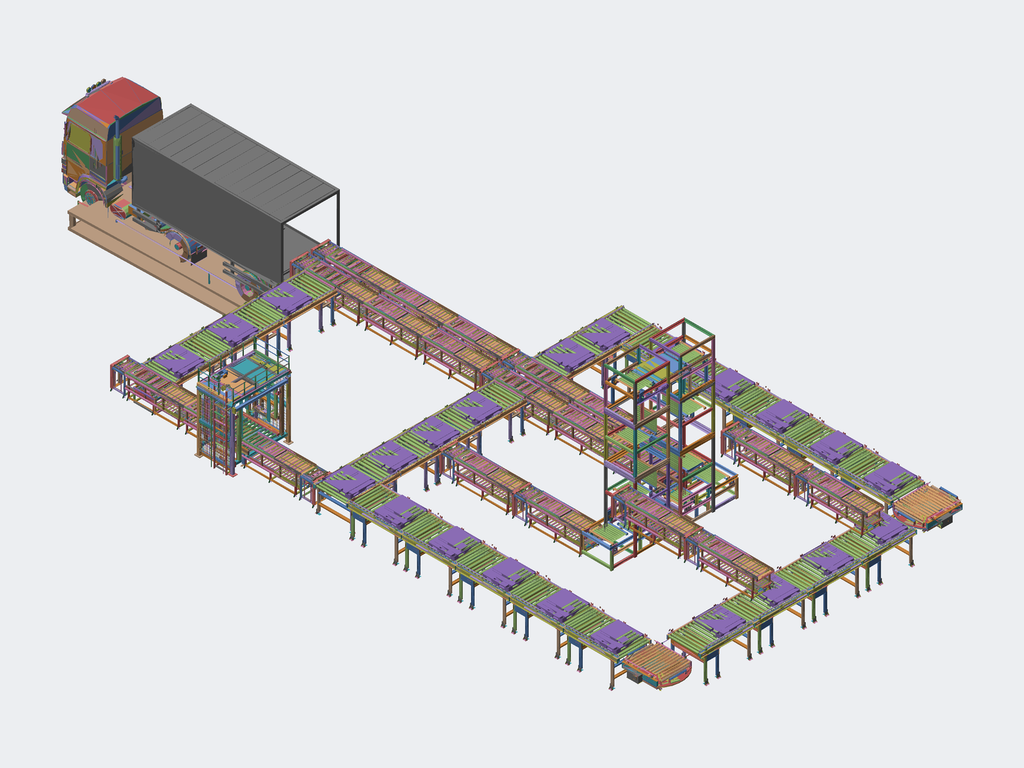Assembly | STEP file | 551 different items | 36567 placed
Parts list (item | name | quantity | parent item | size | volume), first 334 of 551 items:
1 | Sprocket mounting plate XG | x12 | in Single sprocket assembly 1XG(default), Single sprocket assembly 1XG(default)-1, Single sprocket assembly 1XG(default-_flexible1), Single sprocket assembly 1XG(default)-2, Single sprocket assembly 2XG, Single sprocket assembly 2XG-1 | 190 x 350 x 25 mm | 1631084 mm3
2 | 24A16T sprocket XG | x12 | in Single sprocket assembly 1XG(default), Single sprocket assembly 1XG(default)-1, Single sprocket assembly 1XG(default-_flexible1), Single sprocket assembly 1XG(default)-2, Single sprocket assembly 2XG, Single sprocket assembly 2XG-1 | 210 x 210 x 50 mm | 700498 mm3
3 | Single sprocket shaft 1XG | x8 | in Single sprocket assembly 1XG(default), Single sprocket assembly 1XG(default)-1, Single sprocket assembly 1XG(default-_flexible1), Single sprocket assembly 1XG(default)-2 | 50 x 60 x 140 mm | 188778 mm3
4 | 6208 deep groove ball bearing XG | x24 | in Single sprocket assembly 1XG(default), Single sprocket assembly 1XG(default)-1, Single sprocket assembly 1XG(default-_flexible1), Single sprocket assembly 1XG(default)-2, Single sprocket assembly 2XG, Single sprocket assembly 2XG-1 | - | -
5 | Single sprocket shaft end cover 1XG | x12 | in Single sprocket assembly 1XG(default), Single sprocket assembly 1XG(default)-1, Single sprocket assembly 1XG(default-_flexible1), Single sprocket assembly 1XG(default)-2, Single sprocket assembly 2XG, Single sprocket assembly 2XG-1 | 60 x 60 x 10 mm | 27505 mm3
6 | 40 spacer XG | x12 | in Single sprocket assembly 1XG(default), Single sprocket assembly 1XG(default)-1, Single sprocket assembly 1XG(default-_flexible1), Single sprocket assembly 1XG(default)-2, Single sprocket assembly 2XG, Single sprocket assembly 2XG-1 | 70 x 70 x 5 mm | 12959 mm3
7 | Single sprocket shaft 2XG | x4 | in Single sprocket assembly 2XG, Single sprocket assembly 2XG-1 | 80 x 80 x 230 mm | 591587 mm3
8 | Bearing housing mounting plate XG | x12 | in Double sprocket bearing housing assembly 1XG, Double sprocket bearing housing assembly 1XG-1, Double sprocket bearing housing assembly 1XG-2, Double sprocket bearing housing assembly 1XG-3, Double sprocket bearing housing assembly 1XG-4, Double sprocket bearing housing assembly 1XG-5 | 190 x 350 x 25 mm | 1489768 mm3
9 | UCF208 bearing housing XG | x12 | in Double sprocket bearing housing assembly 1XG, Double sprocket bearing housing assembly 1XG-1, Double sprocket bearing housing assembly 1XG-2, Double sprocket bearing housing assembly 1XG-3, Double sprocket bearing housing assembly 1XG-4, Double sprocket bearing housing assembly 1XG-5 | 130 x 130 x 51.2 mm | 310699 mm3
10 | Drive double sprocket shaft 1XG | x4 | in Drive double sprocket assembly 1XG, Drive double sprocket assembly 1XG-1 | 50 x 50 x 1380 mm | 2550231 mm3
11 | 24A16T sprocket 2XG | x24 | in Drive double sprocket assembly 1XG, Double sprocket assembly 1XG, Drive double sprocket assembly 1XG-1 | 210 x 210 x 50 mm | 809619 mm3
12 | 40 bushing | x12 | in Drive double sprocket assembly 1XG, Double sprocket assembly 1XG, Drive double sprocket assembly 1XG-1 | 90 x 90 x 40 mm | 139406 mm3
13 | Double sprocket shaft 1XG | x2 | in Double sprocket assembly 1XG | 50 x 50 x 1320 mm | 2495026 mm3
14 | Outer chain 1XG | x4 | in Outer chain assembly 1XG, Outer chain assembly 1XG-1 | - | 6318542 mm3
15 | Outer chain 1-1XG | x4 | in Outer chain assembly 1XG, Outer chain assembly 1XG-1 | - | 4555438 mm3
16 | Inner chain 1XG | x4 | in Inner chain assembly 1XG, Inner chain assembly 1XG-1 | - | 4855051 mm3
17 | Inner chain 1-1XG | x4 | in Inner chain assembly 1XG, Inner chain assembly 1XG-1 | - | 4555438 mm3
18 | 24A double-side double-hole chain 1 | x420 | in Double-side double-hole chain assembly 1, Double-side double-hole chain assembly 1-1, Double-side double-hole chain assembly 1-2, Double-side double-hole chain assembly 1-3, Double-side double-hole chain assembly 1-4, Double-side double-hole chain assembly 1-5, Double-side double-hole chain assembly 1-6, Double-side double-hole chain assembly 1-7, Double-side double-hole chain assembly 1-8, Double-side double-hole chain assembly 1-9, Double-side double-hole chain assembly 1-10, Double-side double-hole chain assembly 1-11, Double-side double-hole chain assembly 1-12, Double-side double-hole chain assembly 1-13, Double-side double-hole chain assembly 1-14, Double-side double-hole chain assembly 1-15, Double-side double-hole chain assembly 1-16, Double-side double-hole chain assembly 1-17, Double-side double-hole chain assembly 1-18, Double-side double-hole chain assembly 1-19, Double-side double-hole chain assembly 1-20 | 68 x 38 x 99 mm | 48081 mm3
19 | 24A double-side double-hole chain 2 | x378 | in Double-side double-hole chain assembly 1, Double-side double-hole chain assembly 1-1, Double-side double-hole chain assembly 1-2, Double-side double-hole chain assembly 1-3, Double-side double-hole chain assembly 1-4, Double-side double-hole chain assembly 1-5, Double-side double-hole chain assembly 1-6, Double-side double-hole chain assembly 1-7, Double-side double-hole chain assembly 1-8, Double-side double-hole chain assembly 1-9, Double-side double-hole chain assembly 1-10, Double-side double-hole chain assembly 1-11, Double-side double-hole chain assembly 1-12, Double-side double-hole chain assembly 1-13, Double-side double-hole chain assembly 1-14, Double-side double-hole chain assembly 1-15, Double-side double-hole chain assembly 1-16, Double-side double-hole chain assembly 1-17, Double-side double-hole chain assembly 1-18, Double-side double-hole chain assembly 1-19, Double-side double-hole chain assembly 1-20 | 73 x 35 x 35 mm | 33789 mm3
20 | Rear link plate | x14 | in Link plate assembly, 链PlateAssembly-1, 链PlateAssembly-2, 链PlateAssembly-3, 链PlateAssembly-4, 链PlateAssembly-5, 链PlateAssembly-6 | 68 x 70 x 1000 mm | 1230922 mm3
21 | Front link plate | x14 | in Link plate assembly, 链PlateAssembly-1, 链PlateAssembly-2, 链PlateAssembly-3, 链PlateAssembly-4, 链PlateAssembly-5, 链PlateAssembly-6 | 68 x 70 x 820 mm | 1047322 mm3
22 | Middle link plate | x112 | in Link plate assembly, 链PlateAssembly-1, 链PlateAssembly-2, 链PlateAssembly-3, 链PlateAssembly-4, 链PlateAssembly-5, 链PlateAssembly-6 | 74 x 15 x 820 mm | 903391 mm3
23 | Conveyor belt bracket | x4 | in Conveyor assembly 1 | 63 x 160 x 1184 mm | 2475798 mm3
24 | Adjusting plate XG | x4 | in Conveyor assembly 1 | 450 x 110 x 10 mm | 387044 mm3
25 | Bearing mounting plate XG | x4 | in Conveyor assembly 1 | 132 x 110 x 25 mm | 218118 mm3
26 | Adjusting plate-1XG | x4 | in Conveyor assembly 1 | 300 x 110 x 55 mm | 464863 mm3
27 | Screw seat XG | x4 | in Conveyor assembly 1 | 90 x 60 x 60 mm | 144633 mm3
28 | Adjusting plate clamp | x4 | in Conveyor assembly 1 | 30 x 110 x 10 mm | 31099 mm3
29 | Bearing housing F206 | x8 | in Conveyor assembly 1 | 106 x 41.5 x 106 mm | 142901 mm3
30 | socket head cap screw_iso(ISO 4762 M10 x 40 - 40N) | x4 | in Conveyor assembly 1 | 50 x 16 x 16 mm | 4794 mm3
31 | Roller XG3 | x2 | in Conveyor assembly 1 | 175 x 250 x 175 mm | 677038 mm3
32 | Roller XG1 | x4 | in Conveyor assembly 1 | 195 x 987 x 195 mm | 5708379 mm3
33 | Roller XG2 | x6 | in Conveyor assembly 1 | 175 x 105 x 175 mm | 577278 mm3
34 | Belt XG | x2 | in Conveyor assembly 1 | 1201 x 201 x 950 mm | 7472801 mm3
35 | Reinforcing rod XG | x4 | in Conveyor assembly 1 | 110 x 1000 x 60 mm | 1058206 mm3
36 | Bracket 1XG(default_machined_) | x2 | in Continuous lifting machine assembly 1XG | 2500 x 1300 x 2850 mm | 65972501 mm3
37 | Bracket 2XG(default_machined_) | x2 | in Continuous lifting machine assembly 1XG | 1500 x 1300 x 1950 mm | 30079515 mm3
38 | Bracket 3XG(default_machined_) | x2 | in Continuous lifting machine assembly 1XG | 2400 x 1300 x 1700 mm | 40025813 mm3
39 | circlips for shaft--type a large gb(GB_CONNECTING_PIECE_RING_RRA 30) | x2 | in Continuous lifting machine assembly 1XG | 33.5 x 36.571 x 1.2 mm | 372.611 mm3
40 | Support steel plate | x2 | in Continuous lifting machine assembly 1XG | 880 x 1107 x 15.737 mm | 3066275 mm3
41 | 链轮-1 (1) | x2 | in Continuous lifting machine assembly 1XG | 122.017 x 124.5 x 33 mm | 168369 mm3
42 | 链轮-1 (2) | x2 | in Continuous lifting machine assembly 1XG | 122.017 x 124.5 x 33 mm | 159053 mm3
43 | Plate A | x4 | in Continuous lifting machine assembly 1XG | 100 x 15 x 500 mm | 747549 mm3
44 | Motor mounting plate | x2 | in Continuous lifting machine assembly 1XG | 520 x 20 x 250 mm | 2541854 mm3
45 | hex nuts, style 1-grades ab gb(GB_FASTENER_NUT_SNAB1  B M39-N) | x2 | in Continuous lifting machine assembly 1XG | 69.282 x 60 x 33.4 mm | 71685 mm3
46 | Reinforcing plate | x20 | in Continuous lifting machine assembly 1XG | 190 x 60 x 15 mm | 164161 mm3
47 | 24A16T | x2 | in Continuous lifting machine assembly 1XG | 210 x 210 x 50 mm | 858195 mm3
48 | Motor | x2 | in Continuous lifting machine assembly 1XG | 400 x 310 x 480 mm | 30638928 mm3
49 | 24A16T (motor sprocket) | x2 | in Continuous lifting machine assembly 1XG | 210 x 210 x 50 mm | 787504 mm3
50 | Part 4 | x2 | in Continuous lifting machine assembly 1XG | 88 x 12 x 12 mm | 9838 mm3
51 | Part 1 | x2 | in Continuous lifting machine assembly 1XG | 380 x 645.065 x 135 mm | 686374 mm3
52 | Guard cover 2 | x2 | in Continuous lifting machine assembly 1XG | 412.05 x 170 x 140 mm | 209083 mm3
53 | - | x672 | - | 15.011 x 13 x 4 mm | 430.822 mm3
54 | - | x84 | - | 8 x 25 x 1300 mm | 255560 mm3
55 | - | x672 | - | 8 x 180 x 8 mm | 8853 mm3
56 | - | x672 | - | 30.977 x 24 x 30.977 mm | 8556 mm3
57 | - | x84 | - | 1300 x 25 x 1.5 mm | 48655 mm3
58 | - | x672 | - | 16 x 8.4 x 8.4 mm | 245.575 mm3
59 | - | x42 | in 211 | 40 x 80 x 60 mm | 30008 mm3
60 | - | x42 | in 211 | 46.755 x 43.333 x 7.8 mm | 7112 mm3
61 | slotted cheese head screws with shoulder gb_PreviewCfg | x42 | in 211 | 4.82 x 3.5 x 3.5 mm | 20.801 mm3
62 | - | x84 | in 211 | 7 x 7 x 24 mm | 380.939 mm3
63 | - | x1587 | in 211, Double-layer roller line + lifting mechanism | 13 x 33 x 13 mm | 2112 mm3
64 | - | x1290 | in 211, Double-layer roller line + lifting mechanism | 10 x 10 x 30 mm | 2637 mm3
65 | - | x84 | - | 8 x 25 x 1000 mm | 195560 mm3
66 | - | x84 | - | 1000 x 25 x 1.5 mm | 37405 mm3
67 | 2-1 | x42 | - | 51 x 93 x 26 mm | 74170 mm3
68 | 2-2 | x42 | - | 5 x 5 x 5 mm | 86.524 mm3
69 | 2-3 | x42 | - | 5 x 5 x 5 mm | 86.524 mm3
70 | 2-4 | x42 | - | 5 x 5 x 5 mm | 86.524 mm3
71 | 2-5 | x42 | - | 5 x 5 x 5 mm | 86.524 mm3
72 | 2-6 | x42 | - | 5 x 5 x 5 mm | 86.524 mm3
73 | 2-7 | x42 | - | 5 x 5 x 5 mm | 86.524 mm3
74 | 2-8 | x42 | - | 28 x 4 x 4.6 mm | 365.402 mm3
75 | 2-9 | x42 | - | 28 x 4 x 4.6 mm | 365.402 mm3
76 | 2-10 | x42 | - | 48.5 x 80 x 22 mm | 21918 mm3
77 | - | x105 | - | 45 x 738 x 45 mm | 510078 mm3
78 | - | x42 | - | 45 x 150 x 8 mm | 48733 mm3
79 | - | x42 | - | 35 x 562 x 10 mm | 195044 mm3
80 | - | x168 | - | 16 x 10 x 10 mm | 398.324 mm3
81 | - | x84 | - | 45 x 1022 x 45 mm | 707174 mm3
82 | - | x174 | - | 80 x 170 x 38 mm | 57410 mm3
83 | - | x126 | - | 45 x 267.5 x 45 mm | 185188 mm3
84 | NFJN12_100.stp | x174 | - | 128 x 60 x 60 mm | 48974 mm3
85 | - | x168 | - | 45 x 445 x 45 mm | 308069 mm3
86 | - | x84 | - | 45 x 2481 x 45 mm | 1717571 mm3
87 | - | x192 | - | 45 x 45 x 4 mm | 8069 mm3
88 | - | x189 | - | 45 x 658 x 45 mm | 455527 mm3
89 | 50x1.5B_1200-1 | x42 | in 1.100.NHC.BCC-200W | 50 x 50 x 197.6 mm | 45172 mm3
90 | 12C_A-1 | x42 | in 1.100.NHC.BCC-200W | 12 x 12 x 211 mm | 22253 mm3
91 | - | x84 | in 1.100.NHC.BCC-200W | 15.973 x 48.6 x 48.6 mm | 7087 mm3
92 | - | x21 | in 229 | 80 x 100 x 110 mm | 51569 mm3
93 | - | x21 | in 229 | 85 x 100 x 110 mm | 52819 mm3
94 | 1 | x23 | in MGPM20-20Z-M9PL_0_0_0_, Slewing bearing | 36 x 83 x 57 mm | 129991 mm3
95 | 2 | x23 | in MGPM20-20Z-M9PL_0_0_0_, Slewing bearing | 30 x 81 x 64.5 mm | 36360 mm3
96 | 3 | x21 | in MGPM20-20Z-M9PL_0_0_0_ | 4.6 x 4 x 28 mm | 365.402 mm3
97 | 4_1 | x21 | in MGPM20-20Z-M9PL_0_0_0_ | 4.6 x 4 x 28 mm | 365.402 mm3
98 | 5 | x21 | in MGPM20-20Z-M9PL_0_0_0_ | 9.728 x 6.2 x 9.728 mm | 415.838 mm3
99 | 6 | x21 | in MGPM20-20Z-M9PL_0_0_0_ | 9.728 x 6.2 x 9.728 mm | 415.838 mm3
100 | - | x21 | - | 726 x 60 x 5 mm | 213262 mm3
101 | - | x147 | - | 97.772 x 70.687 x 35 mm | 5397 mm3
102 | - | x159 | - | - | -
103 | AS2201F-01-06 | x42 | - | 14.2 x 35.2 x 27.5 mm | 4409 mm3
104 | - | x21 | - | 35 x 81 x 18 mm | 27056 mm3
105 | - | x21 | - | 726 x 30 x 5 mm | 106619 mm3
106 | - | x750 | - | - | -
107 | - | x126 | - | - | -
108 | - | x42 | - | 120 x 10 x 1143 mm | 1358326 mm3
109 | - | x21 | - | 1255 x 636 x 1.5 mm | 1086247 mm3
110 | - | x21 | - | 120 x 10 x 1143 mm | 1355255 mm3
111 | - | x21 | - | 120 x 10 x 1143 mm | 1359044 mm3
112 | - | x21 | - | 726 x 60 x 5 mm | 213239 mm3
113 | - | x21 | - | 1234 x 636 x 1.5 mm | 1146720 mm3
114 | - | x42 | - | 120 x 10 x 1346 mm | 1602562 mm3
115 | - | x21 | - | 120 x 10 x 1346 mm | 1594815 mm3
116 | - | x21 | - | 120 x 10 x 1346 mm | 1599795 mm3
117 | - | x84 | - | 118.296 x 125.997 x 10 mm | 10541 mm3
118 | - | x588 | - | 130.012 x 138.996 x 10 mm | 11591 mm3
119 | - | x42 | - | 207.005 x 98.34 x 93 mm | 532374 mm3
120 | - | x42 | - | 103 x 165.5 x 15 mm | 204204 mm3
121 | - | x66 | - | 145.075 x 155.71 x 10 mm | 12941 mm3
122 | OP070-1 | x21 | - | 350 x 30 x 550 mm | 865842 mm3
123 | - | x22 | in Pallet depalletizer-palletizer stp | 20 x 174 x 44 mm | 24719 mm3
124 | TWH25-C57-R75-CONNECTION | x216 | in TWH25-C57-R75-26 | 79.373 x 81 x 35 mm | 33777 mm3
125 | TWH25-C57-R75-FIX-END | x12 | in TWH25-C57-R75-26 | - | -
126 | TWH25-C57-R75-FREE-END | x12 | in TWH25-C57-R75-26 | - | -
127 | - | x24 | - | 45 x 757.5 x 45 mm | 524410 mm3
128 | - | x24 | - | 45 x 658 x 45 mm | 455527 mm3
129 | - | x24 | - | 820 x 45 x 90 mm | 1189309 mm3
130 | - | x24 | - | 45 x 476 x 45 mm | 329530 mm3
131 | - | x12 | - | 45 x 820 x 45 mm | 567678 mm3
132 | - | x24 | - | 45 x 517 x 45 mm | 356541 mm3
133 | - | x12 | - | 52 x 27.713 x 24 mm | 12410 mm3
134 | - | x24 | - | 45 x 636 x 45 mm | 440296 mm3
135 | - | x12 | - | 380 x 636 x 15 mm | 2517055 mm3
136 | - | x12 | - | 343.5 x 157 x 122.87 mm | 3393544 mm3
137 | - | x12 | - | 48 x 48 x 16 mm | 14884 mm3
138 | - | x24 | - | 8 x 25 x 430 mm | 80647 mm3
139 | - | x12 | - | 60 x 636 x 80 mm | 212766 mm3
140 | - | x12 | - | 25 x 40 x 60 mm | 5907 mm3
141 | - | x12 | - | 459 x 6 x 135 mm | 364434 mm3
142 | - | x48 | - | 40 x 63 x 100 mm | 17364 mm3
143 | - | x24 | - | 430 x 25 x 1.5 mm | 16066 mm3
144 | - | x12 | - | 30 x 23.12 x 23.12 mm | 4440 mm3
145 | - | x12 | - | 459 x 6 x 135 mm | 364434 mm3
146 | - | x12 | - | 45 x 436.5 x 20 mm | 379711 mm3
147 | - | x24 | - | 90 x 748 x 15 mm | 978302 mm3
148 | - | x24 | - | 20 x 139 x 20 mm | 52128 mm3
149 | - | x12 | - | 820 x 84 x 139 mm | 6920085 mm3
150 | - | x48 | - | 330 x 45 x 10 mm | 141601 mm3
151 | - | x48 | - | 25 x 25 x 670 mm | 328039 mm3
152 | - | x48 | - | 94.752 x 94.752 x 15 mm | 48670 mm3
153 | - | x12 | - | 220 x 134 x 85 mm | 598597 mm3
154 | - | x12 | - | 92.631 x 92.631 x 30 mm | 108519 mm3
155 | - | x12 | - | 75 x 88 x 5 mm | 31916 mm3
156 | - | x12 | - | 50 x 35 x 110 mm | 19995 mm3
157 | - | x12 | - | 50 x 40 x 60 mm | 8457 mm3
158 | - | x24 | - | 90.5 x 40 x 45 mm | 12606 mm3
159 | - | x12 | - | 40 x 40 x 40 mm | 8321 mm3
160 | - | x12 | - | 161.812 x 174.281 x 10 mm | 14441 mm3
161 | - | x12 | - | 90 x 748 x 15 mm | 986342 mm3
162 | - | x24 | - | 105.2 x 31.177 x 27 mm | 31063 mm3
163 | - | x12 | - | 85 x 100 x 15 mm | 114454 mm3
164 | - | x24 | - | 20 x 20 x 96 mm | 29253 mm3
165 | - | x12 | - | 90 x 67 x 30 mm | 152526 mm3
166 | - | x12 | - | 55 x 180 x 130 mm | 251570 mm3
167 | - | x12 | - | 143 x 121 x 12 mm | 171712 mm3
168 | - | x12 | - | 25 x 25 x 45 mm | 12533 mm3
169 | - | x12 | - | 76 x 36 x 15 mm | 18163 mm3
170 | - | x12 | - | 49 x 36 x 36 mm | 41848 mm3
171 | - | x12 | - | 80 x 100 x 10 mm | 76229 mm3
172 | - | x48 | - | 45 x 90 x 5 mm | 19575 mm3
173 | - | x12 | - | 10 x 10 x 12 mm | 362.854 mm3
174 | - | x12 | - | 12 x 12 x 38.7 mm | 3601 mm3
175 | kcmfl-25 | x48 | - | 62 x 62 x 112 mm | 98286 mm3
176 | - | x36 | - | 8.5 x 13 x 8.5 mm | 400.62 mm3
177 | - | x462 | in Double-layer roller line + lifting mechanism | 13 x 38 x 13 mm | 2363 mm3
178 | - | x330 | in Double-layer roller line + lifting mechanism | 13 x 24 x 13 mm | 1660 mm3
179 | - | x99 | in Double-layer roller line + lifting mechanism | 20 x 16.428 x 16.428 mm | 1361 mm3
180 | - | x275 | in Double-layer roller line + lifting mechanism | 13 x 28 x 13 mm | 1861 mm3
181 | - | x44 | in Double-layer roller line + lifting mechanism | 13 x 68 x 13 mm | 3871 mm3
182 | - | x11 | in Double-layer roller line + lifting mechanism | 10 x 26 x 10 mm | 933.458 mm3
183 | - | x44 | in Double-layer roller line + lifting mechanism | 30 x 25.075 x 25.075 mm | 4579 mm3
184 | - | x66 | in Double-layer roller line + lifting mechanism | 12 x 10 x 10 mm | 319.784 mm3
185 | - | x176 | in Double-layer roller line + lifting mechanism | 8.5 x 30 x 8.5 mm | 734.47 mm3
186 | - | x88 | in Double-layer roller line + lifting mechanism | 20 x 12.399 x 12.399 mm | 709.68 mm3
187 | - | x44 | in Double-layer roller line + lifting mechanism | 16 x 90 x 16 mm | 7923 mm3
188 | - | x66 | in Double-layer roller line + lifting mechanism | 35 x 12.399 x 12.399 mm | 1134 mm3
189 | - | x110 | in Double-layer roller line + lifting mechanism | 35 x 25.075 x 25.075 mm | 5144 mm3
190 | - | x66 | in Double-layer roller line + lifting mechanism | 13 x 43 x 13 mm | 2615 mm3
191 | - | x264 | in Double-layer roller line + lifting mechanism | 10 x 16 x 10 mm | 650.705 mm3
192 | - | x44 | in Double-layer roller line + lifting mechanism | 12 x 8.4 x 8.4 mm | 195.31 mm3
193 | - | x10 | - | 186.5 x 75 x 75 mm | 216850 mm3
194 | - | x10 | - | 226 x 62.5 x 62.5 mm | 136978 mm3
195 | - | x10 | - | 8 x 26.558 x 23 mm | 2309 mm3
196 | SC63_752 | x40 | - | 156.5 x 12 x 12 mm | 7243 mm3
197 | JSI63_2 | x40 | - | 21.5 x 12 x 12 mm | 1588 mm3
198 | 63_C_Screw | x20 | - | 17.1 x 10 x 10 mm | 818.333 mm3
199 | Outer_ring_gear_1 | x20 | - | 1.224 x 10 x 9.485 mm | 14.03 mm3
200 | F_M16150U_F-M16150U-P | x10 | - | 40 x 22 x 84 mm | 29098 mm3
201 | F_SC63CA_F-SC63CA | x10 | - | 46.5 x 74 x 74 mm | 62495 mm3
202 | F_SC63CB_F-SC63CB | x10 | - | 31.5 x 74 x 74 mm | 67976 mm3
203 | PDR30_part | x40 | in PDR30_PDR30, PDR30_PDR30-1, PDR30_PDR30-2, PDR30_PDR30-3, PDR30_PDR30-4, PDR30_PDR30-5, PDR30_PDR30-6, PDR30_PDR30-7 | 165 x 91 x 48 mm | 216054 mm3
204 | PDR30_set_screw | x80 | in PDR30_PDR30, PDR30_PDR30-1, PDR30_PDR30-2, PDR30_PDR30-3, PDR30_PDR30-4, PDR30_PDR30-5, PDR30_PDR30-6, PDR30_PDR30-7 | 5 x 6 x 6 mm | 118.771 mm3
205 | - | x40 | - | 150 x 150 x 8 mm | 108756 mm3
206 | - | x10 | - | 50 x 55 x 720 mm | 407064 mm3
207 | - | x20 | - | 30.311 x 35 x 90.5 mm | 47417 mm3
208 | circlips for shaft--type a large gb_PreviewCfg | x20 | - | 11.5 x 13.997 x 1 mm | 50.603 mm3
209 | angular contact ball bearing_68_iso_ISO 15 ABB - 1020 - Full,DE,AC,Full_68 | x160 | - | 12 x 42 x 42 mm | 8271 mm3
210 | - | x40 | - | 128 x 95 x 71 mm | 210049 mm3
211 | - | x40 | - | 67 x 41.5 x 41.5 mm | 47696 mm3
212 | - | x80 | - | 27 x 27 x 13.5 mm | 3274 mm3
213 | - | x40 | - | 20 x 20 x 150 mm | 42054 mm3
214 | short pitch roller chain wheel_d_iso_Chain wheel ISO - 16Z 10B-2 --16SC50H34L42.0N | x40 | - | 34.001 x 89.463 x 89.463 mm | 79108 mm3
215 | - | x5 | in Lifting transfer machine 1 | 750 x 578 x 945 mm | 6599392 mm3
216 | - | x20 | in Lifting transfer machine 1 | 90 x 85 x 90 mm | 60517 mm3
217 | - | x10 | in Lifting transfer machine 1 | 35 x 35 x 753 mm | 624999 mm3
218 | - | x20 | in Lifting transfer machine 1 | 40 x 40 x 8 mm | 7406 mm3
219 | - | x20 | in Lifting transfer machine 1 | 50 x 200 x 8 mm | 66352 mm3
220 | - | x5 | in Lifting transfer machine 1 | 626 x 970 x 110 mm | 2991413 mm3
221 | - | x20 | in Lifting transfer machine 1 | 38.947 x 38.288 x 90.5 mm | 66959 mm3
222 | - | x20 | in Lifting transfer machine 1 | 150 x 140.041 x 660 mm | 992784 mm3
223 | - | x20 | in Lifting transfer machine 1 | 41 x 12 x 620 mm | 198150 mm3
224 | - | x30 | in Lifting transfer machine 1 | 12 x 12 x 320 mm | 33018 mm3
225 | hex nut gradec_iso_Hexagon Nut ISO - 4034 - M12 - N | x30 | in Lifting transfer machine 1 | 18.001 x 20.785 x 12.2 mm | 2393 mm3
226 | - | x5 | in Lifting transfer machine 1 | 35 x 35 x 1052 mm | 947063 mm3
227 | short pitch roller chain wheel_s_iso_Chain wheel ISO - 14Z 10A-1 --14SB50H40L25.0N | x5 | in Lifting transfer machine 1 | 40.001 x 79.165 x 81.025 mm | 73610 mm3
228 | short pitch roller chain wheel_d_iso_Chain wheel ISO - 16Z 10B-2 --16SB60H50L30.0R1 | x10 | in Lifting transfer machine 1 | 50.001 x 89.463 x 89.463 mm | 141597 mm3
229 | - | x10 | in Lifting transfer machine 1 | 180 x 155 x 68 mm | 262430 mm3
230 | - | x10 | in Lifting transfer machine 1 | 142 x 83 x 42.2 mm | 151622 mm3
231 | R37DT71D4 | x5 | in Lifting transfer machine 1 | 251.513 x 122.1 x 91.448 mm | 1177142 mm3
232 | 1-Base_default<welded> | x2 | in 001-Base assembly | 1030 x 50 x 1030 mm | 12734708 mm3
233 | 2-Foot seat_default<welded> | x8 | in 001-Base assembly | 100 x 50 x 80 mm | 109934 mm3
234 | BASE_Foot_GFTR16-100-100 | x8 | in Foot_GFTR16-100-100 | 100 x 150 x 100 mm | 177771 mm3
235 | NAT_Foot_GFTR16-100-100 | x8 | in Foot_GFTR16-100-100 | 24 x 9 x 27.403 mm | 3116 mm3
236 | 3-Motor plate | x2 | in 001-Base assembly | 220 x 10 x 142 mm | 292914 mm3
237 | 4-Rotating drive shaft | x2 | in 001-Base assembly | 186 x 40 x 40 mm | 107459 mm3
238 | Spur gear_GearTrax | x2 | in 001-Base assembly | 169.505 x 169.505 x 50 mm | 949713 mm3
239 | RV025-090_063.step_1 | x4 | in RVFF025-090 worm gear reducer_063_25_FA_P71B14_F4_ZB_b01 | 112 x 174 x 148 mm | 1644542 mm3
240 | Output hollow shaft_063_25.step_1 | x4 | in RVFF025-090 worm gear reducer_063_25_FA_P71B14_F4_ZB_b01 | 42.5 x 42.5 x 112 mm | 100706 mm3
241 | Bearing sleeve_063_25.step_1 | x4 | in RVFF025-090 worm gear reducer_063_25_FA_P71B14_F4_ZB_b01 | 70 x 70 x 112 mm | 272052 mm3
242 | Input motor flange_063_P71B14.step | x4 | in RVFF025-090 worm gear reducer_063_25_FA_P71B14_F4_ZB_b01 | 105 x 105 x 21 mm | 72142 mm3
243 | Output flange_063_ZB.step_1 | x4 | in RVFF025-090 worm gear reducer_063_25_FA_P71B14_F4_ZB_b01 | 142 x 142 x 50 mm | 173016 mm3
244 | Motor_P71B14.step | x4 | in RVFF025-090 worm gear reducer_063_25_FA_P71B14_F4_ZB_b01 | 138 x 162 x 247 mm | 2733778 mm3
245 | 5-Slewing support plate | x2 | in 002-Support frame | 600 x 10 x 600 mm | 2301617 mm3
246 | 6-Slewing support rod_default<machined> | x12 | in 002-Support frame | 140 x 40 x 150 mm | 106539 mm3
247 | 16-Photoeye mounting plate | x2 | in 002-Support frame | 75 x 25 x 20 mm | 5163 mm3
248 | FC-SPX303Z | x2 | in 002-Support frame | 26 x 26.2 x 13.7 mm | 2282 mm3
249 | 7-Roller base_default<machined> | x2 | in 003-Roller section | 2105 x 48 x 1497 mm | 25567908 mm3
250 | 8-Body driven side | x2 | in 003-Roller section | 40 x 189 x 1480 mm | 1252545 mm3
251 | 9-Body drive side_default<machined> | x2 | in 003-Roller section | 60 x 179.5 x 1480 mm | 1116104 mm3
252 | 5分-13齿双排滚筒_GearTrax | x24 | in 003-Roller section | 76.009 x 76 x 1490 mm | 6520792 mm3
253 | 5-fen-13-tooth_GearTrax | x2 | in 003-Roller section | 75.004 x 75.553 x 24.975 mm | 40881 mm3
254 | 10-Roller motor plate | x2 | in 003-Roller section | 253 x 130 x 46.5 mm | 181020 mm3
255 | 11-Unpowered roller support plate | x16 | in 003-Roller section | 60 x 174 x 70 mm | 89255 mm3
256 | φ76-1200 | x4 | in 003-Roller section | 1200 x 76 x 76 mm | 5359963 mm3
257 | φ76-700 | x4 | in 003-Roller section | 700 x 76 x 76 mm | 3091733 mm3
258 | 12-Chain cover plate | x2 | in 003-Roller section | 1480 x 44 x 69 mm | 341077 mm3
259 | 13-Guardrail bracket | x8 | in 003-Roller section | 30 x 75 x 80 mm | 78230 mm3
260 | 14-Guardrail_default<machined> | x4 | in 003-Roller section | 1571 x 32 x 316 mm | 277538 mm3
261 | 15-Roller drive shaft | x2 | in 003-Roller section | 215 x 25 x 25 mm | 100964 mm3
262 | 17-Detection plate_default<machined> | x2 | in 003-Roller section | 310.044 x 125 x 310.044 mm | 48050 mm3
263 | 18-Top post_default<machined> | x2 | in 003-Roller section | 220 x 20 x 120 mm | 67083 mm3
264 | 20-Motor cover | x2 | in 003-Roller section | 537 x 270 x 180 mm | 476658 mm3
265 | 21-Motor cover plate | x2 | in 003-Roller section | 25 x 181 x 482 mm | 105638 mm3
266 | 22-Cover plate | x2 | in 003-Roller section | 680 x 2 x 680 mm | 924081 mm3
267 | 19-Limit post | x4 | in 000-Main assembly | 55 x 40 x 55 mm | 86991 mm3
268 | KS D 3568 - 100 x 50 x 3.2 - 940 | x23 | in Frame 1712202625821 | 50 x 100 x 940 mm | 830002 mm3
269 | KS D 3568 - 100 x 50 x 3.2 - 940_1 | x23 | in Frame 1712202625821 | 50 x 100 x 940 mm | 829758 mm3
270 | KS D 3568 - 100 x 50 x 3.2 - 1350 | x23 | in Frame 1712202625821 | 50 x 100 x 1350 mm | 1193238 mm3
271 | KS D 3568 - 100 x 50 x 3.2 - 940_2 | x23 | in Frame 1712202625821 | 50 x 100 x 940 mm | 830002 mm3
272 | KS D 3568 - 100 x 50 x 3.2 - 400 | x23 | in Frame 1712202625821 | 50 x 100 x 400 mm | 353552 mm3
273 | KS D 3568 - 100 x 50 x 3.2 - 940_3 | x23 | in Frame 1712202625821 | 50 x 100 x 940 mm | 829758 mm3
274 | KS D 3568 - 100 x 50 x 3.2 - 1350_1 | x23 | in Frame 1712202625821 | 50 x 100 x 1350 mm | 1193238 mm3
275 | DCV-000-006 | x23 | in DCV-000-W06-940H | 440 x 160 x 15 mm | 1014226 mm3
276 | DCV-000-026 | x138 | in DCV-000-W06-940H, DCV-000-W07-940H | 190 x 50 x 9 mm | 83111 mm3
277 | DCV-000-025 | x138 | in DCV-000-W06-940H, DCV-000-W07-940H | 100 x 50 x 16 mm | 75363 mm3
278 | DCV-000-027 | x138 | in DCV-000-W06-940H, DCV-000-W07-940H | 80 x 90 x 9 mm | 63615 mm3
279 | DCV-000-022 | x138 | in DCV-000-W08 | 120 x 80 x 12 mm | 112838 mm3
280 | DCV-000-021 | x138 | in DCV-000-W08 | 120 x 180 x 12 mm | 238691 mm3
281 | DCV-000-023 | x276 | in DCV-000-W08 | 50 x 70 x 12 mm | 27000 mm3
282 | DCV-000-024 | x138 | in DCV-000-A08 | 100 x 100 x 5 mm | 49571 mm3
283 | MF64-M20-100_1 | x138 | in MF64-M20-100 | 64 x 132 x 64 mm | 83393 mm3
284 | KS B 1012 - M 20 | x138 | in MF64-M20-100 | 16 x 34.641 x 30 mm | 8623 mm3
285 | DCV-000-005 | x23 | in DCV-000-A06-940H | 380 x 160 x 15 mm | 876589 mm3
286 | RPH_0.75KW (1_30) | x23 | in DCV-000-A06-940H | - | -
287 | DCV-000-004 | x23 | in DCV-000-A06-940H | 35 x 73.041 x 73.574 mm | 55395 mm3
288 | DCV-000-028 | x23 | in DCV-000-A06-940H | 34 x 34 x 4.5 mm | 3658 mm3
289 | DCV-000-010 | x23 | in DCV-000-A06-940H | 470 x 217 x 5 mm | 507673 mm3
290 | DCV-000-011 | x46 | in DCV-000-A06-940H | 1450 x 256 x 20 mm | 581295 mm3
291 | KS B 1326 - 8x15.5 | x115 | in DCV-000-A06-940H | 1.6 x 15.5 x 15.5 mm | 213.239 mm3
292 | KS B 1324 - No. 2 - 8 | x115 | in DCV-000-A06-940H | 2 x 14.6 x 14.6 mm | 224.071 mm3
293 | KS B 1002 - C  M 8 x 20 | x23 | in DCV-000-A06-940H | 25.3 x 15.011 x 13 mm | 1773 mm3
294 | KS B 1002 - C  M 8 x 80 | x46 | in DCV-000-A06-940H | 85.3 x 15.011 x 13 mm | 4789 mm3
295 | KS B 1012 - M 8 | x46 | in DCV-000-A06-940H | 6.5 x 15.011 x 13 mm | 715.11 mm3
296 | KS B 1326 - 6x11.5 | x644 | in DCV-000-A06-940H, DCV-000-A05-2300L | 1.6 x 11.5 x 11.5 mm | 114.718 mm3
297 | KS B 1324 - No. 2 - 6 | x414 | in DCV-000-A06-940H | 1.5 x 11.5 x 11.5 mm | 109.527 mm3
298 | KS B 1002 - C  M 6 x 16 | x368 | in DCV-000-A06-940H | 20 x 11.547 x 10 mm | 794.666 mm3
299 | KS B 1326 - 10x18 | x1334 | in DCV-000-A06-940H, DCV-000-A05-2300L, DCV-000-A07-940H, Single-layer roller conveyor line | 2 x 18 x 18 mm | 335.758 mm3
300 | KS B 1324 - No. 2 - 10 | x920 | in DCV-000-A06-940H, DCV-000-A05-2300L, DCV-000-A07-940H, Single-layer roller conveyor line | 2.5 x 17.6 x 17.6 mm | 394.643 mm3
301 | KS B 1002 - C  M 10 x 30 | x276 | in DCV-000-A06-940H, DCV-000-A07-940H | 36.4 x 18.475 x 16 mm | 3759 mm3
302 | FITTING-UNION-10AxD12 | x23 | in DCV-000-A06-940H | 31.1 x 20.5 x 20.5 mm | 6256 mm3
303 | FITTING-ELBOW-10A | x23 | in DCV-000-A06-940H | 17.46 x 40.703 x 36.281 mm | 10729 mm3
304 | TUBE-STS | x23 | in DCV-000-A06-940H | 9.52 x 104.76 x 104.76 mm | 5600 mm3
305 | FITTING-UNION-10Ax10A | x23 | in DCV-000-A06-940H | 39.153 x 25 x 21.651 mm | 8100 mm3
306 | SUCPP10A | x23 | in DCV-000-A06-940H | 16.949 x 21 x 16.949 mm | 2402 mm3
307 | DCV-000-012 | x23 | in DCV-000-A06-940H | 150 x 34 x 10 mm | 49407 mm3
308 | KS B 1002 - C  M 6 x 25 | x46 | in DCV-000-A06-940H | 29 x 11.547 x 10 mm | 1049 mm3
309 | KS B 1002 - C  M 8 x 30 | x92 | in DCV-000-A06-940H | 35.3 x 15.011 x 13 mm | 2275 mm3
310 | KS B 1002 - C  M 10 x 35 | x92 | in DCV-000-A06-940H | 41.4 x 18.475 x 16 mm | 4152 mm3
311 | DCV-000-038 | x23 | in DCV-000-A06-940H | 233.4 x 210 x 63 mm | 105230 mm3
312 | DCV-000-038_MIR | x23 | in DCV-000-A06-940H | 233.4 x 210 x 63 mm | 105230 mm3
313 | DCV-000-030-2291L | x23 | in DCV-000-W04-2300L | 2291 x 165 x 50 mm | 2555022 mm3
314 | DCV-000-013-B | x46 | in DCV-000-W04-2300L | 107.5 x 165 x 4.5 mm | 65667 mm3
315 | DCV-000-031-2291L | x23 | in DCV-000-W05-2300L | 2300 x 165 x 50 mm | 2571604 mm3
316 | DCV-000-014-B | x46 | in DCV-000-W05-2300L | 156 x 45.5 x 4.5 mm | 30798 mm3
317 | DCV-000-001 | x368 | in DCV-000-W01 | 1270 x 76.3 x 76.3 mm | 923470 mm3
318 | DCV-000-002 | x368 | in DCV-000-W01 | 79.7 x 73.041 x 73.574 mm | 132681 mm3
319 | DCV-000-003 | x368 | in DCV-000-W01 | 72 x 72 x 25 mm | 61649 mm3
320 | DCV-000-009 | x46 | in DCV-000-A01 | 1354 x 20 x 20 mm | 419638 mm3
321 | KS B 2023 - 6004 - 20 x 42 x 12 | x736 | in DCV-000-A01, DCV-000-A02 | 12 x 42 x 42 mm | 8691 mm3
322 | KS B 1336 - 20 x 1.2 | x736 | in DCV-000-A01, DCV-000-A02 | 24.05 x 26.087 x 1.2 mm | 211.892 mm3
323 | KS B 1336 - 42x1.8 | x368 | in DCV-000-A01, DCV-000-A02 | 44.5 x 43.174 x 1.8 mm | 686.31 mm3
324 | KS B 1336 - 47x1.8 | x368 | in DCV-000-A01, DCV-000-A02 | 49.5 x 48.026 x 1.8 mm | 847.052 mm3
325 | KS B 2023 - 6204 - 20 x 47 x 14 | x368 | in DCV-000-A01, DCV-000-A02 | 14 x 47 x 47 mm | 13264 mm3
326 | DCV-000-008 | x322 | in DCV-000-A02 | 1350 x 20 x 20 mm | 418627 mm3
327 | DCV-000-W02_1 | x23 | in DCV-000-W02 | 9 x 4.5 x 50 mm | 434.569 mm3
328 | DCV-000-018 | x23 | in DCV-000-W02 | 9 x 9 x 220 mm | 5529 mm3
329 | DCV-000-016 | x23 | in DCV-000-W02 | 35 x 55 x 20 mm | 6902 mm3
330 | E3Z-R61 5M_PART1 | x23 | in E3Z-R61 5M | 24.985 x 38.085 x 10.8 mm | 6468 mm3
331 | DCV-000-020 | x46 | in DCV-000-A03, DCV-000-A04 | 38 x 30 x 35 mm | 29966 mm3
332 | KS B 1028 - Flat point M6x10 | x184 | in DCV-000-A03, DCV-000-A04 | 10 x 6 x 6 mm | 245.798 mm3
333 | KS B 1326 - 5x10 | x253 | in DCV-000-A03, DCV-000-A04, DCV-000-A05-2300L | 1 x 10 x 10 mm | 56.478 mm3
334 | KS B 1324 - No. 2 - 5 | x92 | in DCV-000-A03, DCV-000-A04 | 1.3 x 8.5 x 8.5 mm | 46.057 mm3
Placements (level | parent | child | x y z in mm | rotation matrix by rows), first 171 of 39055 lines:
1 | 座椅输送线布局3D-2026.01.15 | Continuous lifting machine assembly 1XG | 7711.575 418.464 -5262.009 | 0 -1 0 1 0 0 0 0 1
2 | Continuous lifting machine assembly 1XG | Single sprocket assembly 1XG(default) | -57.73 733.718 7141.467 | 1 0 0 0 0 -1 0 1 0
3 | Single sprocket assembly 1XG(default) | Sprocket mounting plate XG | -23.725 8.533 300.0 | 1 0 0 0 1 0 0 0 1
3 | Single sprocket assembly 1XG(default) | 24A16T sprocket XG | -23.725 8.533 385.0 | 1 0.003815 0 -0.003815 1 0 0 0 1
3 | Single sprocket assembly 1XG(default) | Single sprocket shaft 1XG | -23.725 8.533 385.0 | -0.8716 -0.4903 0 -0.4903 0.8716 0 0 0 -1
3 | Single sprocket assembly 1XG(default) | 6208 deep groove ball bearing XG | -23.725 8.533 344.0 | -0.8977 -0.4407 0 -0.4407 0.8977 0 0 0 -1
3 | Single sprocket assembly 1XG(default) | 6208 deep groove ball bearing XG | -23.725 8.533 376.0 | 0.998 0.0632 0 -0.0632 0.998 0 0 0 1
3 | Single sprocket assembly 1XG(default) | Single sprocket shaft end cover 1XG | -23.725 8.533 385.0 | 0.8716 -0.4903 0 0.4903 0.8716 0 0 0 1
3 | Single sprocket assembly 1XG(default) | 40 spacer XG | -23.725 8.533 295.0 | 1 0 0 0 1 0 0 0 1
2 | Continuous lifting machine assembly 1XG | Single sprocket assembly 1XG(default)-1 | -105.18 -1066.282 7141.467 | -1 0 0 0 0 1 0 1 -0
3 | Single sprocket assembly 1XG(default)-1 | Sprocket mounting plate XG | -23.725 8.533 300.0 | 1 0 0 0 1 0 0 0 1
3 | Single sprocket assembly 1XG(default)-1 | 24A16T sprocket XG | -23.725 8.533 385.0 | 1 0.003815 0 -0.003815 1 0 0 0 1
3 | Single sprocket assembly 1XG(default)-1 | Single sprocket shaft 1XG | -23.725 8.533 385.0 | -0.8716 -0.4903 0 -0.4903 0.8716 0 0 0 -1
3 | Single sprocket assembly 1XG(default)-1 | 6208 deep groove ball bearing XG | -23.725 8.533 344.0 | -0.8977 -0.4407 0 -0.4407 0.8977 0 0 0 -1
3 | Single sprocket assembly 1XG(default)-1 | 6208 deep groove ball bearing XG | -23.725 8.533 376.0 | 0.998 0.0632 0 -0.0632 0.998 0 0 0 1
3 | Single sprocket assembly 1XG(default)-1 | Single sprocket shaft end cover 1XG | -23.725 8.533 385.0 | 0.8716 -0.4903 0 0.4903 0.8716 0 0 0 1
3 | Single sprocket assembly 1XG(default)-1 | 40 spacer XG | -23.725 8.533 295.0 | 1 0 0 0 1 0 0 0 1
2 | Continuous lifting machine assembly 1XG | Single sprocket assembly 1XG(default-_flexible1) | -252.73 733.718 2286.467 | 1 0 0 0 0 -1 0 1 -0
3 | Single sprocket assembly 1XG(default-_flexible1) | Sprocket mounting plate XG | -23.725 8.533 300.0 | 1 0 0 0 1 0 0 0 1
3 | Single sprocket assembly 1XG(default-_flexible1) | 24A16T sprocket XG | -23.725 8.533 385.0 | 0.0166 -0.9999 0 0.9999 0.0166 0 0 0 1
3 | Single sprocket assembly 1XG(default-_flexible1) | Single sprocket shaft 1XG | -23.725 8.533 385.0 | -0.8716 -0.4903 0 -0.4903 0.8716 0 0 0 -1
3 | Single sprocket assembly 1XG(default-_flexible1) | 6208 deep groove ball bearing XG | -23.725 8.533 376.0 | 0.998 0.0632 0 -0.0632 0.998 0 0 0 1
3 | Single sprocket assembly 1XG(default-_flexible1) | 6208 deep groove ball bearing XG | -23.725 8.533 344.0 | -0.8977 -0.4407 0 -0.4407 0.8977 0 0 0 -1
3 | Single sprocket assembly 1XG(default-_flexible1) | Single sprocket shaft end cover 1XG | -23.725 8.533 385.0 | 0.8716 -0.4903 0 0.4903 0.8716 0 0 0 1
3 | Single sprocket assembly 1XG(default-_flexible1) | 40 spacer XG | -23.725 8.533 295.0 | 1 0 0 0 1 0 0 0 1
2 | Continuous lifting machine assembly 1XG | Single sprocket assembly 1XG(default)-2 | -300.18 -1066.282 2286.467 | -1 0 0 0 0 1 0 1 0
3 | Single sprocket assembly 1XG(default)-2 | Sprocket mounting plate XG | -23.725 8.533 300.0 | 1 0 0 0 1 0 0 0 1
3 | Single sprocket assembly 1XG(default)-2 | 24A16T sprocket XG | -23.725 8.533 385.0 | 1 0.003815 0 -0.003815 1 0 0 0 1
3 | Single sprocket assembly 1XG(default)-2 | Single sprocket shaft 1XG | -23.725 8.533 385.0 | -0.8716 -0.4903 0 -0.4903 0.8716 0 0 0 -1
3 | Single sprocket assembly 1XG(default)-2 | 6208 deep groove ball bearing XG | -23.725 8.533 344.0 | -0.8977 -0.4407 0 -0.4407 0.8977 0 0 0 -1
3 | Single sprocket assembly 1XG(default)-2 | 6208 deep groove ball bearing XG | -23.725 8.533 376.0 | 0.998 0.0632 0 -0.0632 0.998 0 0 0 1
3 | Single sprocket assembly 1XG(default)-2 | Single sprocket shaft end cover 1XG | -23.725 8.533 385.0 | 0.8716 -0.4903 0 0.4903 0.8716 0 0 0 1
3 | Single sprocket assembly 1XG(default)-2 | 40 spacer XG | -23.725 8.533 295.0 | 1 0 0 0 1 0 0 0 1
2 | Continuous lifting machine assembly 1XG | Single sprocket assembly 2XG | 402.55 168.718 2291.629 | -1 0 0 0 0 1 0 1 0
3 | Single sprocket assembly 2XG | Sprocket mounting plate XG | -4.995 3.371 240.0 | 1 0 0 0 1 0 0 0 1
3 | Single sprocket assembly 2XG | 24A16T sprocket XG | -4.995 3.371 90.0 | -0.9925 -0.1219 0 -0.1219 0.9925 0 0 0 -1
3 | Single sprocket assembly 2XG | 6208 deep groove ball bearing XG | -4.995 3.371 99.0 | -0.9237 -0.383 0 -0.383 0.9237 0 0 0 -1
3 | Single sprocket assembly 2XG | 6208 deep groove ball bearing XG | -4.995 3.371 131.0 | 1 0 0 0 1 0 0 0 1
3 | Single sprocket assembly 2XG | Single sprocket shaft end cover 1XG | -4.995 3.371 80.0 | 1 0 0 0 1 0 0 0 1
3 | Single sprocket assembly 2XG | 40 spacer XG | -4.995 3.371 265.0 | 1 0 0 0 1 0 0 0 1
3 | Single sprocket assembly 2XG | Single sprocket shaft 2XG | -4.995 3.371 90.0 | 1 0 0 0 1 0 0 0 1
2 | Continuous lifting machine assembly 1XG | Single sprocket assembly 2XG-1 | 412.54 -501.282 2291.629 | 1 0 0 0 0 -1 0 1 -0
3 | Single sprocket assembly 2XG-1 | Sprocket mounting plate XG | -4.995 3.371 240.0 | 1 0 0 0 1 0 0 0 1
3 | Single sprocket assembly 2XG-1 | 24A16T sprocket XG | -4.995 3.371 90.0 | -0.9925 -0.1219 0 -0.1219 0.9925 0 0 0 -1
3 | Single sprocket assembly 2XG-1 | 6208 deep groove ball bearing XG | -4.995 3.371 99.0 | -0.9237 -0.383 0 -0.383 0.9237 0 0 0 -1
3 | Single sprocket assembly 2XG-1 | 6208 deep groove ball bearing XG | -4.995 3.371 131.0 | 1 0 0 0 1 0 0 0 1
3 | Single sprocket assembly 2XG-1 | Single sprocket shaft end cover 1XG | -4.995 3.371 80.0 | 1 0 0 0 1 0 0 0 1
3 | Single sprocket assembly 2XG-1 | 40 spacer XG | -4.995 3.371 265.0 | 1 0 0 0 1 0 0 0 1
3 | Single sprocket assembly 2XG-1 | Single sprocket shaft 2XG | -4.995 3.371 90.0 | 1 0 0 0 1 0 0 0 1
2 | Continuous lifting machine assembly 1XG | Double sprocket bearing housing assembly 1XG | 608.788 121.218 7174.765 | 1 0 0 0 0 1 0 -1 0
3 | Double sprocket bearing housing assembly 1XG | Bearing housing mounting plate XG | -6.243 24.765 287.5 | 1 0 0 0 1 0 0 0 1
3 | Double sprocket bearing housing assembly 1XG | UCF208 bearing housing XG | -6.243 24.765 320.0 | 1 0 0 0 1 0 0 0 1
2 | Continuous lifting machine assembly 1XG | Double sprocket bearing housing assembly 1XG-1 | 596.302 -453.782 7174.765 | -1 0 0 0 0 -1 0 -1 -0
3 | Double sprocket bearing housing assembly 1XG-1 | Bearing housing mounting plate XG | -6.243 24.765 287.5 | 1 0 0 0 1 0 0 0 1
3 | Double sprocket bearing housing assembly 1XG-1 | UCF208 bearing housing XG | -6.243 24.765 320.0 | 1 0 0 0 1 0 0 0 1
2 | Continuous lifting machine assembly 1XG | Drive double sprocket assembly 1XG | 604.445 1133.718 7140.446 | 0.004483 -1 0 0 0 -1 1 0.004483 -0
3 | Drive double sprocket assembly 1XG | Drive double sprocket shaft 1XG | 9.545 1.942 1300.0 | 1 0 0 0 1 0 0 0 1
3 | Drive double sprocket assembly 1XG | 24A16T sprocket 2XG | 9.545 1.942 785.0 | 0 1 0 -1 0 0 0 0 1
3 | Drive double sprocket assembly 1XG | 24A16T sprocket 2XG | 9.545 1.942 875.0 | 0 1 0 -1 0 0 0 0 1
3 | Drive double sprocket assembly 1XG | 24A16T sprocket 2XG | 9.545 1.942 1725.0 | 0 1 0 1 0 0 0 0 -1
3 | Drive double sprocket assembly 1XG | 24A16T sprocket 2XG | 9.545 1.942 1815.0 | 0 1 0 1 0 0 0 0 -1
3 | Drive double sprocket assembly 1XG | 40 bushing | 9.545 1.942 1795.0 | 0 1 0 -1 0 0 0 0 1
3 | Drive double sprocket assembly 1XG | 40 bushing | 9.545 1.942 805.0 | 0 1 0 -1 0 0 0 0 1
2 | Continuous lifting machine assembly 1XG | Double sprocket bearing housing assembly 1XG-2 | -1223.698 -453.782 2124.765 | -1 0 0 0 0 -1 0 -1 -0
3 | Double sprocket bearing housing assembly 1XG-2 | Bearing housing mounting plate XG | -6.243 24.765 287.5 | 1 0 0 0 1 0 0 0 1
3 | Double sprocket bearing housing assembly 1XG-2 | UCF208 bearing housing XG | -6.243 24.765 320.0 | 1 0 0 0 1 0 0 0 1
2 | Continuous lifting machine assembly 1XG | Double sprocket bearing housing assembly 1XG-3 | -1211.211 121.218 2124.765 | 1 0 0 0 0 1 0 -1 0
3 | Double sprocket bearing housing assembly 1XG-3 | Bearing housing mounting plate XG | -6.243 24.765 287.5 | 1 0 0 0 1 0 0 0 1
3 | Double sprocket bearing housing assembly 1XG-3 | UCF208 bearing housing XG | -6.243 24.765 320.0 | 1 0 0 0 1 0 0 0 1
2 | Continuous lifting machine assembly 1XG | Double sprocket assembly 1XG | -1219.421 1193.718 2099.422 | 0.7139 0.7002 0 0 0 -1 -0.7002 0.7139 -0
3 | Double sprocket assembly 1XG | 24A16T sprocket 2XG | 0.9989 1.79 935.0 | 0 1 0 -1 0 0 0 0 1
3 | Double sprocket assembly 1XG | 24A16T sprocket 2XG | 0.9989 1.79 1785.0 | 0 1 0 1 0 0 0 0 -1
3 | Double sprocket assembly 1XG | 24A16T sprocket 2XG | 0.9989 1.79 845.0 | 0 1 0 -1 0 0 0 0 1
3 | Double sprocket assembly 1XG | 24A16T sprocket 2XG | 0.9989 1.79 1875.0 | 0 1 0 1 0 0 0 0 -1
3 | Double sprocket assembly 1XG | 40 bushing | 0.9989 1.79 1855.0 | 0 1 0 -1 0 0 0 0 1
3 | Double sprocket assembly 1XG | 40 bushing | 0.9989 1.79 865.0 | 0 1 0 -1 0 0 0 0 1
3 | Double sprocket assembly 1XG | Double sprocket shaft 1XG | 0.9989 1.79 1360.0 | 1 0 0 0 1 0 0 0 1
2 | Continuous lifting machine assembly 1XG | Double sprocket bearing housing assembly 1XG-4 | 596.302 -453.782 2124.765 | -1 0 0 0 0 -1 0 -1 -0
3 | Double sprocket bearing housing assembly 1XG-4 | Bearing housing mounting plate XG | -6.243 24.765 287.5 | 1 0 0 0 1 0 0 0 1
3 | Double sprocket bearing housing assembly 1XG-4 | UCF208 bearing housing XG | -6.243 24.765 320.0 | 1 0 0 0 1 0 0 0 1
2 | Continuous lifting machine assembly 1XG | Double sprocket bearing housing assembly 1XG-5 | 608.788 121.218 2124.765 | 1 0 0 0 0 1 0 -1 0
3 | Double sprocket bearing housing assembly 1XG-5 | Bearing housing mounting plate XG | -6.243 24.765 287.5 | 1 0 0 0 1 0 0 0 1
3 | Double sprocket bearing housing assembly 1XG-5 | UCF208 bearing housing XG | -6.243 24.765 320.0 | 1 0 0 0 1 0 0 0 1
2 | Continuous lifting machine assembly 1XG | Drive double sprocket assembly 1XG-1 | 606.011 1133.718 2090.897 | -0.1623 -0.9867 0 0 0 -1 0.9867 -0.1623 0
3 | Drive double sprocket assembly 1XG-1 | Drive double sprocket shaft 1XG | 9.545 1.942 1300.0 | 1 0 0 0 1 0 0 0 1
3 | Drive double sprocket assembly 1XG-1 | 24A16T sprocket 2XG | 9.545 1.942 785.0 | 0 1 0 -1 0 0 0 0 1
3 | Drive double sprocket assembly 1XG-1 | 24A16T sprocket 2XG | 9.545 1.942 1815.0 | 0 1 0 1 0 0 0 0 -1
3 | Drive double sprocket assembly 1XG-1 | 24A16T sprocket 2XG | 9.545 1.942 875.0 | 0 1 0 -1 0 0 0 0 1
3 | Drive double sprocket assembly 1XG-1 | 24A16T sprocket 2XG | 9.545 1.942 1725.0 | 0 1 0 1 0 0 0 0 -1
3 | Drive double sprocket assembly 1XG-1 | 40 bushing | 9.545 1.942 1795.0 | 0 1 0 -1 0 0 0 0 1
3 | Drive double sprocket assembly 1XG-1 | 40 bushing | 9.545 1.942 805.0 | 0 1 0 -1 0 0 0 0 1
2 | Continuous lifting machine assembly 1XG | Outer chain assembly 1XG | -206.078 5641.716 4600.102 | 1 0 0 0 0 -1 0 1 -0
3 | Outer chain assembly 1XG | Outer chain 1XG | -1011.377 -2500.102 5281.497 | 1 0 0 0 1 0 0 0 1
3 | Outer chain assembly 1XG | Outer chain 1-1XG | -1011.377 -2500.102 5281.497 | 1 0 0 0 1 0 0 0 1
2 | Continuous lifting machine assembly 1XG | Outer chain assembly 1XG-1 | -206.078 4588.716 4600.102 | 1 0 0 0 0 -1 0 1 0
3 | Outer chain assembly 1XG-1 | Outer chain 1XG | -1011.377 -2500.102 5281.497 | 1 0 0 0 1 0 0 0 1
3 | Outer chain assembly 1XG-1 | Outer chain 1-1XG | -1011.377 -2500.102 5281.497 | 1 0 0 0 1 0 0 0 1
2 | Continuous lifting machine assembly 1XG | Inner chain assembly 1XG | -44.801 5550.58 4350.454 | 1 0 0 0 0 -1 0 1 -0
3 | Inner chain assembly 1XG | Inner chain 1XG | -1172.654 -2250.454 5280.362 | 1 0 0 0 1 0 0 0 1
3 | Inner chain assembly 1XG | Inner chain 1-1XG | -1172.654 -2250.454 5280.362 | 1 0 0 0 1 0 0 0 1
2 | Continuous lifting machine assembly 1XG | Inner chain assembly 1XG-1 | -44.801 4677.58 4350.454 | 1 0 0 0 0 -1 0 1 -0
3 | Inner chain assembly 1XG-1 | Inner chain 1XG | -1172.654 -2250.454 5280.362 | 1 0 0 0 1 0 0 0 1
3 | Inner chain assembly 1XG-1 | Inner chain 1-1XG | -1172.654 -2250.454 5280.362 | 1 0 0 0 1 0 0 0 1
2 | Continuous lifting machine assembly 1XG | Link plate assembly | -1182.236 836.718 2209.149 | 1 0 0 0 0 -1 0 1 0
3 | Link plate assembly | Double-side double-hole chain assembly 1 | -9.22 1.107 904.0 | 1 0 0 0 1 0 0 0 1
4 | Double-side double-hole chain assembly 1 | 24A double-side double-hole chain 1 | 297.001 -0.7558 99.0 | 1 0 0 0 1 0 0 0 1
4 | Double-side double-hole chain assembly 1 | 24A double-side double-hole chain 1 | 525.001 -0.7558 99.0 | 1 0 0 0 1 0 0 0 1
4 | Double-side double-hole chain assembly 1 | 24A double-side double-hole chain 1 | 601.001 -0.7558 99.0 | 1 0 0 0 1 0 0 0 1
4 | Double-side double-hole chain assembly 1 | 24A double-side double-hole chain 1 | 449.001 -0.7558 99.0 | 1 0 0 0 1 0 0 0 1
4 | Double-side double-hole chain assembly 1 | 24A double-side double-hole chain 1 | 677.001 -0.7558 99.0 | 1 0 0 0 1 0 0 0 1
4 | Double-side double-hole chain assembly 1 | 24A double-side double-hole chain 1 | 221.001 -0.7558 99.0 | 1 0 0 0 1 0 0 0 1
4 | Double-side double-hole chain assembly 1 | 24A double-side double-hole chain 1 | 145.001 -0.7558 99.0 | 1 0 0 0 1 0 0 0 1
4 | Double-side double-hole chain assembly 1 | 24A double-side double-hole chain 1 | -6.999 -0.7558 99.0 | 1 0 0 0 1 0 0 0 1
4 | Double-side double-hole chain assembly 1 | 24A double-side double-hole chain 1 | 69.001 -0.7558 99.0 | 1 0 0 0 1 0 0 0 1
4 | Double-side double-hole chain assembly 1 | 24A double-side double-hole chain 1 | 373.001 -0.7558 99.0 | 1 0 0 0 1 0 0 0 1
4 | Double-side double-hole chain assembly 1 | 24A double-side double-hole chain 2 | 487.001 -0.7558 99.0 | 1 0 0 0 1 0 0 0 1
4 | Double-side double-hole chain assembly 1 | 24A double-side double-hole chain 2 | 107.001 -0.7558 99.0 | 1 0 0 0 1 0 0 0 1
4 | Double-side double-hole chain assembly 1 | 24A double-side double-hole chain 2 | 183.001 -0.7558 99.0 | 1 0 0 0 1 0 0 0 1
4 | Double-side double-hole chain assembly 1 | 24A double-side double-hole chain 2 | 411.001 -0.7558 99.0 | 1 0 0 0 1 0 0 0 1
4 | Double-side double-hole chain assembly 1 | 24A double-side double-hole chain 2 | 31.001 -0.7558 99.0 | 1 0 0 0 1 0 0 0 1
4 | Double-side double-hole chain assembly 1 | 24A double-side double-hole chain 2 | 563.001 -0.7558 99.0 | 1 0 0 0 1 0 0 0 1
4 | Double-side double-hole chain assembly 1 | 24A double-side double-hole chain 2 | 639.001 -0.7558 99.0 | 1 0 0 0 1 0 0 0 1
4 | Double-side double-hole chain assembly 1 | 24A double-side double-hole chain 2 | 335.001 -0.7558 99.0 | 1 0 0 0 1 0 0 0 1
4 | Double-side double-hole chain assembly 1 | 24A double-side double-hole chain 2 | 259.001 -0.7558 99.0 | 1 0 0 0 1 0 0 0 1
3 | Link plate assembly | Double-side double-hole chain assembly 1-1 | -9.22 1.107 1204.0 | 1 0 0 0 1 0 0 0 1
4 | Double-side double-hole chain assembly 1-1 | 24A double-side double-hole chain 1 | 525.001 -0.7558 99.0 | 1 0 0 0 1 0 0 0 1
4 | Double-side double-hole chain assembly 1-1 | 24A double-side double-hole chain 1 | 221.001 -0.7558 99.0 | 1 0 0 0 1 0 0 0 1
4 | Double-side double-hole chain assembly 1-1 | 24A double-side double-hole chain 1 | 449.001 -0.7558 99.0 | 1 0 0 0 1 0 0 0 1
4 | Double-side double-hole chain assembly 1-1 | 24A double-side double-hole chain 1 | 69.001 -0.7558 99.0 | 1 0 0 0 1 0 0 0 1
4 | Double-side double-hole chain assembly 1-1 | 24A double-side double-hole chain 1 | 297.001 -0.7558 99.0 | 1 0 0 0 1 0 0 0 1
4 | Double-side double-hole chain assembly 1-1 | 24A double-side double-hole chain 1 | 145.001 -0.7558 99.0 | 1 0 0 0 1 0 0 0 1
4 | Double-side double-hole chain assembly 1-1 | 24A double-side double-hole chain 1 | 601.001 -0.7558 99.0 | 1 0 0 0 1 0 0 0 1
4 | Double-side double-hole chain assembly 1-1 | 24A double-side double-hole chain 1 | 373.001 -0.7558 99.0 | 1 0 0 0 1 0 0 0 1
4 | Double-side double-hole chain assembly 1-1 | 24A double-side double-hole chain 1 | -6.999 -0.7558 99.0 | 1 0 0 0 1 0 0 0 1
4 | Double-side double-hole chain assembly 1-1 | 24A double-side double-hole chain 1 | 677.001 -0.7558 99.0 | 1 0 0 0 1 0 0 0 1
4 | Double-side double-hole chain assembly 1-1 | 24A double-side double-hole chain 2 | 335.001 -0.7558 99.0 | 1 0 0 0 1 0 0 0 1
4 | Double-side double-hole chain assembly 1-1 | 24A double-side double-hole chain 2 | 183.001 -0.7558 99.0 | 1 0 0 0 1 0 0 0 1
4 | Double-side double-hole chain assembly 1-1 | 24A double-side double-hole chain 2 | 639.001 -0.7558 99.0 | 1 0 0 0 1 0 0 0 1
4 | Double-side double-hole chain assembly 1-1 | 24A double-side double-hole chain 2 | 31.001 -0.7558 99.0 | 1 0 0 0 1 0 0 0 1
4 | Double-side double-hole chain assembly 1-1 | 24A double-side double-hole chain 2 | 107.001 -0.7558 99.0 | 1 0 0 0 1 0 0 0 1
4 | Double-side double-hole chain assembly 1-1 | 24A double-side double-hole chain 2 | 487.001 -0.7558 99.0 | 1 0 0 0 1 0 0 0 1
4 | Double-side double-hole chain assembly 1-1 | 24A double-side double-hole chain 2 | 259.001 -0.7558 99.0 | 1 0 0 0 1 0 0 0 1
4 | Double-side double-hole chain assembly 1-1 | 24A double-side double-hole chain 2 | 563.001 -0.7558 99.0 | 1 0 0 0 1 0 0 0 1
4 | Double-side double-hole chain assembly 1-1 | 24A double-side double-hole chain 2 | 411.001 -0.7558 99.0 | 1 0 0 0 1 0 0 0 1
3 | Link plate assembly | Double-side double-hole chain assembly 1-2 | -9.22 1.107 604.0 | 1 0 0 0 1 0 0 0 1
4 | Double-side double-hole chain assembly 1-2 | 24A double-side double-hole chain 1 | 525.001 -0.7558 99.0 | 1 0 0 0 1 0 0 0 1
4 | Double-side double-hole chain assembly 1-2 | 24A double-side double-hole chain 1 | 145.001 -0.7558 99.0 | 1 0 0 0 1 0 0 0 1
4 | Double-side double-hole chain assembly 1-2 | 24A double-side double-hole chain 1 | 373.001 -0.7558 99.0 | 1 0 0 0 1 0 0 0 1
4 | Double-side double-hole chain assembly 1-2 | 24A double-side double-hole chain 1 | 449.001 -0.7558 99.0 | 1 0 0 0 1 0 0 0 1
4 | Double-side double-hole chain assembly 1-2 | 24A double-side double-hole chain 1 | 69.001 -0.7558 99.0 | 1 0 0 0 1 0 0 0 1
4 | Double-side double-hole chain assembly 1-2 | 24A double-side double-hole chain 1 | 297.001 -0.7558 99.0 | 1 0 0 0 1 0 0 0 1
4 | Double-side double-hole chain assembly 1-2 | 24A double-side double-hole chain 1 | 601.001 -0.7558 99.0 | 1 0 0 0 1 0 0 0 1
4 | Double-side double-hole chain assembly 1-2 | 24A double-side double-hole chain 1 | 677.001 -0.7558 99.0 | 1 0 0 0 1 0 0 0 1
4 | Double-side double-hole chain assembly 1-2 | 24A double-side double-hole chain 1 | -6.999 -0.7558 99.0 | 1 0 0 0 1 0 0 0 1
4 | Double-side double-hole chain assembly 1-2 | 24A double-side double-hole chain 1 | 221.001 -0.7558 99.0 | 1 0 0 0 1 0 0 0 1
4 | Double-side double-hole chain assembly 1-2 | 24A double-side double-hole chain 2 | 411.001 -0.7558 99.0 | 1 0 0 0 1 0 0 0 1
4 | Double-side double-hole chain assembly 1-2 | 24A double-side double-hole chain 2 | 335.001 -0.7558 99.0 | 1 0 0 0 1 0 0 0 1
4 | Double-side double-hole chain assembly 1-2 | 24A double-side double-hole chain 2 | 31.001 -0.7558 99.0 | 1 0 0 0 1 0 0 0 1
4 | Double-side double-hole chain assembly 1-2 | 24A double-side double-hole chain 2 | 487.001 -0.7558 99.0 | 1 0 0 0 1 0 0 0 1
4 | Double-side double-hole chain assembly 1-2 | 24A double-side double-hole chain 2 | 183.001 -0.7558 99.0 | 1 0 0 0 1 0 0 0 1
4 | Double-side double-hole chain assembly 1-2 | 24A double-side double-hole chain 2 | 107.001 -0.7558 99.0 | 1 0 0 0 1 0 0 0 1
4 | Double-side double-hole chain assembly 1-2 | 24A double-side double-hole chain 2 | 563.001 -0.7558 99.0 | 1 0 0 0 1 0 0 0 1
4 | Double-side double-hole chain assembly 1-2 | 24A double-side double-hole chain 2 | 259.001 -0.7558 99.0 | 1 0 0 0 1 0 0 0 1
4 | Double-side double-hole chain assembly 1-2 | 24A double-side double-hole chain 2 | 639.001 -0.7558 99.0 | 1 0 0 0 1 0 0 0 1
3 | Link plate assembly | Rear link plate | -16.219 3.351 1003.0 | 1 0 0 0 1 0 0 0 1
3 | Link plate assembly | Front link plate | 667.781 3.351 1003.0 | 1 0 0 0 1 0 0 0 1
3 | Link plate assembly | Middle link plate | 135.781 23.351 1003.0 | 1 0 0 0 1 0 0 0 1
3 | Link plate assembly | Middle link plate | 591.781 23.351 1003.0 | 1 0 0 0 1 0 0 0 1
3 | Link plate assembly | Middle link plate | 363.781 23.351 1003.0 | 1 0 0 0 1 0 0 0 1
3 | Link plate assembly | Middle link plate | 439.781 23.351 1003.0 | 1 0 0 0 1 0 0 0 1
3 | Link plate assembly | Middle link plate | 287.781 23.351 1003.0 | 1 0 0 0 1 0 0 0 1